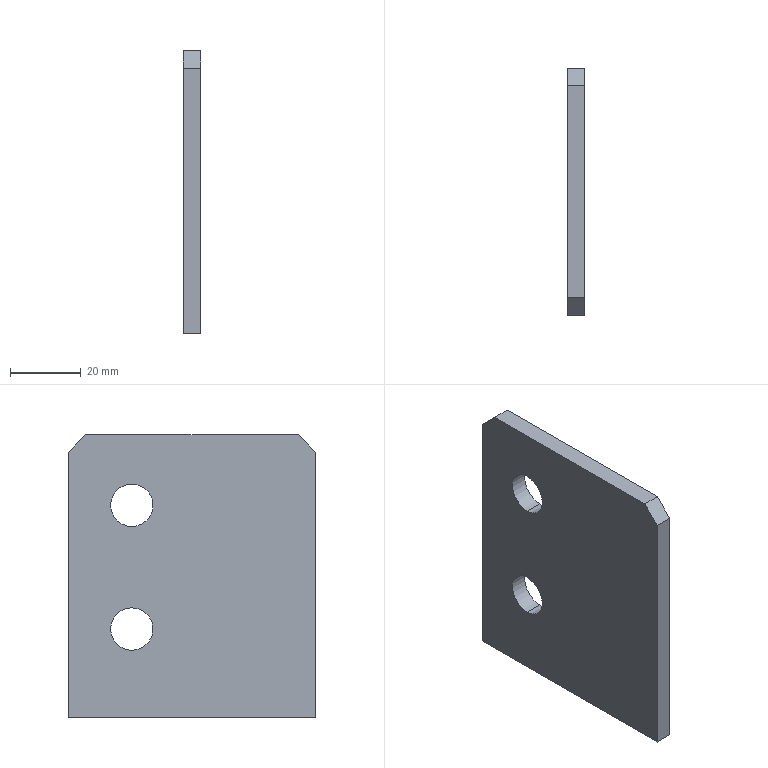Part | STEP file | 1 solid | 12 faces | box 5 x 70 x 80 mm | volume 26744 mm3 | plane 8 | cylinder 4 | commonest cylinder face diameters 12 x4
STEP:
#1=CARTESIAN_POINT('',(0.,0.,0.));
#2=DIRECTION('',(0.,0.,1.));
#3=DIRECTION('',(1.,0.,0.));
#4=AXIS2_PLACEMENT_3D('',#1,#2,#3);
#5=CARTESIAN_POINT('',(165.,97.,31.));
#6=VERTEX_POINT('',#5);
#7=CARTESIAN_POINT('',(165.,97.,19.));
#8=VERTEX_POINT('',#7);
#9=CARTESIAN_POINT('',(165.,97.,25.));
#10=DIRECTION('',(-1.,0.,0.));
#11=DIRECTION('',(0.,0.,1.));
#12=AXIS2_PLACEMENT_3D('',#9,#10,#11);
#13=CIRCLE('',#12,6.);
#14=CARTESIAN_POINT('',(165.,115.,80.));
#15=DIRECTION('',(-1.,0.,0.));
#16=DIRECTION('',(0.,0.,1.));
#17=AXIS2_PLACEMENT_3D('',#14,#15,#16);
#18=PLANE('',#17);
#19=CARTESIAN_POINT('',(-55.,-18.));
#20=DIRECTION('',(1.,0.));
#21=AXIS2_PLACEMENT_2D('',#19,#20);
#22=CIRCLE('',#21,6.);
#23=(GEOMETRIC_REPRESENTATION_CONTEXT(2)PARAMETRIC_REPRESENTATION_CONTEXT()REPRESENTATION_CONTEXT('',''));
#24=DEFINITIONAL_REPRESENTATION('',(#22),#23);
#25=PCURVE('',#18,#24);
#26=CARTESIAN_POINT('',(160.,97.,25.));
#27=DIRECTION('',(-1.,0.,0.));
#28=DIRECTION('',(0.,0.,1.));
#29=AXIS2_PLACEMENT_3D('',#26,#27,#28);
#30=CYLINDRICAL_SURFACE('',#29,6.);
#31=CARTESIAN_POINT('',(0.,-5.));
#32=DIRECTION('',(1.,0.));
#33=VECTOR('',#32,1.);
#34=LINE('',#31,#33);
#35=(GEOMETRIC_REPRESENTATION_CONTEXT(2)PARAMETRIC_REPRESENTATION_CONTEXT()REPRESENTATION_CONTEXT('',''));
#36=DEFINITIONAL_REPRESENTATION('',(#34),#35);
#37=PCURVE('',#30,#36);
#38=SURFACE_CURVE('',#13,(#25,#37),.PCURVE_S1.);
#39=EDGE_CURVE('',#6,#8,#38,.T.);
#40=ORIENTED_EDGE('',*,*,#39,.T.);
#41=CARTESIAN_POINT('',(165.,97.,25.));
#42=DIRECTION('',(-1.,0.,0.));
#43=DIRECTION('',(0.,0.,1.));
#44=AXIS2_PLACEMENT_3D('',#41,#42,#43);
#45=CIRCLE('',#44,6.);
#46=CARTESIAN_POINT('',(-55.,-18.));
#47=DIRECTION('',(1.,0.));
#48=AXIS2_PLACEMENT_2D('',#46,#47);
#49=CIRCLE('',#48,6.);
#50=(GEOMETRIC_REPRESENTATION_CONTEXT(2)PARAMETRIC_REPRESENTATION_CONTEXT()REPRESENTATION_CONTEXT('',''));
#51=DEFINITIONAL_REPRESENTATION('',(#49),#50);
#52=PCURVE('',#18,#51);
#53=CARTESIAN_POINT('',(160.,97.,25.));
#54=DIRECTION('',(-1.,0.,0.));
#55=DIRECTION('',(0.,0.,1.));
#56=AXIS2_PLACEMENT_3D('',#53,#54,#55);
#57=CYLINDRICAL_SURFACE('',#56,6.);
#58=CARTESIAN_POINT('',(0.,-5.));
#59=DIRECTION('',(1.,0.));
#60=VECTOR('',#59,1.);
#61=LINE('',#58,#60);
#62=(GEOMETRIC_REPRESENTATION_CONTEXT(2)PARAMETRIC_REPRESENTATION_CONTEXT()REPRESENTATION_CONTEXT('',''));
#63=DEFINITIONAL_REPRESENTATION('',(#61),#62);
#64=PCURVE('',#57,#63);
#65=SURFACE_CURVE('',#45,(#52,#64),.PCURVE_S1.);
#66=EDGE_CURVE('',#8,#6,#65,.T.);
#67=ORIENTED_EDGE('',*,*,#66,.T.);
#68=EDGE_LOOP('',(#40,#67));
#69=FACE_BOUND('',#68,.T.);
#70=CARTESIAN_POINT('',(165.,97.,66.));
#71=VERTEX_POINT('',#70);
#72=CARTESIAN_POINT('',(165.,97.,54.));
#73=VERTEX_POINT('',#72);
#74=CARTESIAN_POINT('',(165.,97.,60.));
#75=DIRECTION('',(-1.,0.,0.));
#76=DIRECTION('',(0.,0.,1.));
#77=AXIS2_PLACEMENT_3D('',#74,#75,#76);
#78=CIRCLE('',#77,6.);
#79=CARTESIAN_POINT('',(-20.,-18.));
#80=DIRECTION('',(1.,0.));
#81=AXIS2_PLACEMENT_2D('',#79,#80);
#82=CIRCLE('',#81,6.);
#83=(GEOMETRIC_REPRESENTATION_CONTEXT(2)PARAMETRIC_REPRESENTATION_CONTEXT()REPRESENTATION_CONTEXT('',''));
#84=DEFINITIONAL_REPRESENTATION('',(#82),#83);
#85=PCURVE('',#18,#84);
#86=CARTESIAN_POINT('',(160.,97.,60.));
#87=DIRECTION('',(-1.,0.,0.));
#88=DIRECTION('',(0.,0.,1.));
#89=AXIS2_PLACEMENT_3D('',#86,#87,#88);
#90=CYLINDRICAL_SURFACE('',#89,6.);
#91=CARTESIAN_POINT('',(0.,-5.));
#92=DIRECTION('',(1.,0.));
#93=VECTOR('',#92,1.);
#94=LINE('',#91,#93);
#95=(GEOMETRIC_REPRESENTATION_CONTEXT(2)PARAMETRIC_REPRESENTATION_CONTEXT()REPRESENTATION_CONTEXT('',''));
#96=DEFINITIONAL_REPRESENTATION('',(#94),#95);
#97=PCURVE('',#90,#96);
#98=SURFACE_CURVE('',#78,(#85,#97),.PCURVE_S1.);
#99=EDGE_CURVE('',#71,#73,#98,.T.);
#100=ORIENTED_EDGE('',*,*,#99,.T.);
#101=CARTESIAN_POINT('',(165.,97.,60.));
#102=DIRECTION('',(-1.,0.,0.));
#103=DIRECTION('',(0.,0.,1.));
#104=AXIS2_PLACEMENT_3D('',#101,#102,#103);
#105=CIRCLE('',#104,6.);
#106=CARTESIAN_POINT('',(-20.,-18.));
#107=DIRECTION('',(1.,0.));
#108=AXIS2_PLACEMENT_2D('',#106,#107);
#109=CIRCLE('',#108,6.);
#110=(GEOMETRIC_REPRESENTATION_CONTEXT(2)PARAMETRIC_REPRESENTATION_CONTEXT()REPRESENTATION_CONTEXT('',''));
#111=DEFINITIONAL_REPRESENTATION('',(#109),#110);
#112=PCURVE('',#18,#111);
#113=CARTESIAN_POINT('',(160.,97.,60.));
#114=DIRECTION('',(-1.,0.,0.));
#115=DIRECTION('',(0.,0.,1.));
#116=AXIS2_PLACEMENT_3D('',#113,#114,#115);
#117=CYLINDRICAL_SURFACE('',#116,6.);
#118=CARTESIAN_POINT('',(0.,-5.));
#119=DIRECTION('',(1.,0.));
#120=VECTOR('',#119,1.);
#121=LINE('',#118,#120);
#122=(GEOMETRIC_REPRESENTATION_CONTEXT(2)PARAMETRIC_REPRESENTATION_CONTEXT()REPRESENTATION_CONTEXT('',''));
#123=DEFINITIONAL_REPRESENTATION('',(#121),#122);
#124=PCURVE('',#117,#123);
#125=SURFACE_CURVE('',#105,(#112,#124),.PCURVE_S1.);
#126=EDGE_CURVE('',#73,#71,#125,.T.);
#127=ORIENTED_EDGE('',*,*,#126,.T.);
#128=EDGE_LOOP('',(#100,#127));
#129=FACE_BOUND('',#128,.T.);
#130=CARTESIAN_POINT('',(165.,45.,75.));
#131=VERTEX_POINT('',#130);
#132=CARTESIAN_POINT('',(165.,50.,80.));
#133=VERTEX_POINT('',#132);
#134=CARTESIAN_POINT('',(165.,50.,80.));
#135=DIRECTION('',(0.,0.7071,0.7071));
#136=VECTOR('',#135,1.);
#137=LINE('',#134,#136);
#138=CARTESIAN_POINT('',(0.,-65.));
#139=DIRECTION('',(0.7071,0.7071));
#140=VECTOR('',#139,1.);
#141=LINE('',#138,#140);
#142=(GEOMETRIC_REPRESENTATION_CONTEXT(2)PARAMETRIC_REPRESENTATION_CONTEXT()REPRESENTATION_CONTEXT('',''));
#143=DEFINITIONAL_REPRESENTATION('',(#141),#142);
#144=PCURVE('',#18,#143);
#145=CARTESIAN_POINT('',(0.,50.,80.));
#146=DIRECTION('',(0.,-0.7071,0.7071));
#147=DIRECTION('',(-1.,0.,0.));
#148=AXIS2_PLACEMENT_3D('',#145,#146,#147);
#149=PLANE('',#148);
#150=CARTESIAN_POINT('',(-165.,0.));
#151=DIRECTION('',(0.,-1.));
#152=VECTOR('',#151,1.);
#153=LINE('',#150,#152);
#154=(GEOMETRIC_REPRESENTATION_CONTEXT(2)PARAMETRIC_REPRESENTATION_CONTEXT()REPRESENTATION_CONTEXT('',''));
#155=DEFINITIONAL_REPRESENTATION('',(#153),#154);
#156=PCURVE('',#149,#155);
#157=SURFACE_CURVE('',#137,(#144,#156),.PCURVE_S1.);
#158=EDGE_CURVE('',#131,#133,#157,.T.);
#159=ORIENTED_EDGE('',*,*,#158,.F.);
#160=CARTESIAN_POINT('',(165.,45.,0.));
#161=VERTEX_POINT('',#160);
#162=CARTESIAN_POINT('',(165.,45.,80.));
#163=DIRECTION('',(0.,0.,-1.));
#164=VECTOR('',#163,1.);
#165=LINE('',#162,#164);
#166=CARTESIAN_POINT('',(0.,-70.));
#167=DIRECTION('',(-1.,0.));
#168=VECTOR('',#167,1.);
#169=LINE('',#166,#168);
#170=(GEOMETRIC_REPRESENTATION_CONTEXT(2)PARAMETRIC_REPRESENTATION_CONTEXT()REPRESENTATION_CONTEXT('',''));
#171=DEFINITIONAL_REPRESENTATION('',(#169),#170);
#172=PCURVE('',#18,#171);
#173=CARTESIAN_POINT('',(160.,45.,80.));
#174=DIRECTION('',(0.,1.,0.));
#175=DIRECTION('',(1.,0.,0.));
#176=AXIS2_PLACEMENT_3D('',#173,#174,#175);
#177=PLANE('',#176);
#178=CARTESIAN_POINT('',(5.,0.));
#179=DIRECTION('',(0.,1.));
#180=VECTOR('',#179,1.);
#181=LINE('',#178,#180);
#182=(GEOMETRIC_REPRESENTATION_CONTEXT(2)PARAMETRIC_REPRESENTATION_CONTEXT()REPRESENTATION_CONTEXT('',''));
#183=DEFINITIONAL_REPRESENTATION('',(#181),#182);
#184=PCURVE('',#177,#183);
#185=SURFACE_CURVE('',#165,(#172,#184),.PCURVE_S1.);
#186=EDGE_CURVE('',#131,#161,#185,.T.);
#187=ORIENTED_EDGE('',*,*,#186,.T.);
#188=CARTESIAN_POINT('',(165.,115.,0.));
#189=VERTEX_POINT('',#188);
#190=CARTESIAN_POINT('',(165.,0.,0.));
#191=DIRECTION('',(0.,1.,0.));
#192=VECTOR('',#191,1.);
#193=LINE('',#190,#192);
#194=CARTESIAN_POINT('',(-80.,-115.));
#195=DIRECTION('',(0.,1.));
#196=VECTOR('',#195,1.);
#197=LINE('',#194,#196);
#198=(GEOMETRIC_REPRESENTATION_CONTEXT(2)PARAMETRIC_REPRESENTATION_CONTEXT()REPRESENTATION_CONTEXT('',''));
#199=DEFINITIONAL_REPRESENTATION('',(#197),#198);
#200=PCURVE('',#18,#199);
#201=CARTESIAN_POINT('',(0.,0.,0.));
#202=DIRECTION('',(0.,0.,1.));
#203=DIRECTION('',(1.,0.,0.));
#204=AXIS2_PLACEMENT_3D('',#201,#202,#203);
#205=PLANE('',#204);
#206=CARTESIAN_POINT('',(165.,0.));
#207=DIRECTION('',(0.,1.));
#208=VECTOR('',#207,1.);
#209=LINE('',#206,#208);
#210=(GEOMETRIC_REPRESENTATION_CONTEXT(2)PARAMETRIC_REPRESENTATION_CONTEXT()REPRESENTATION_CONTEXT('',''));
#211=DEFINITIONAL_REPRESENTATION('',(#209),#210);
#212=PCURVE('',#205,#211);
#213=SURFACE_CURVE('',#193,(#200,#212),.PCURVE_S1.);
#214=EDGE_CURVE('',#161,#189,#213,.T.);
#215=ORIENTED_EDGE('',*,*,#214,.T.);
#216=CARTESIAN_POINT('',(165.,115.,75.));
#217=VERTEX_POINT('',#216);
#218=CARTESIAN_POINT('',(165.,115.,80.));
#219=DIRECTION('',(0.,0.,1.));
#220=VECTOR('',#219,1.);
#221=LINE('',#218,#220);
#222=CARTESIAN_POINT('',(0.,0.));
#223=DIRECTION('',(1.,0.));
#224=VECTOR('',#223,1.);
#225=LINE('',#222,#224);
#226=(GEOMETRIC_REPRESENTATION_CONTEXT(2)PARAMETRIC_REPRESENTATION_CONTEXT()REPRESENTATION_CONTEXT('',''));
#227=DEFINITIONAL_REPRESENTATION('',(#225),#226);
#228=PCURVE('',#18,#227);
#229=CARTESIAN_POINT('',(160.,115.,80.));
#230=DIRECTION('',(0.,-1.,0.));
#231=DIRECTION('',(0.,0.,-1.));
#232=AXIS2_PLACEMENT_3D('',#229,#230,#231);
#233=PLANE('',#232);
#234=CARTESIAN_POINT('',(0.,5.));
#235=DIRECTION('',(-1.,0.));
#236=VECTOR('',#235,1.);
#237=LINE('',#234,#236);
#238=(GEOMETRIC_REPRESENTATION_CONTEXT(2)PARAMETRIC_REPRESENTATION_CONTEXT()REPRESENTATION_CONTEXT('',''));
#239=DEFINITIONAL_REPRESENTATION('',(#237),#238);
#240=PCURVE('',#233,#239);
#241=SURFACE_CURVE('',#221,(#228,#240),.PCURVE_S1.);
#242=EDGE_CURVE('',#189,#217,#241,.T.);
#243=ORIENTED_EDGE('',*,*,#242,.T.);
#244=CARTESIAN_POINT('',(165.,110.,80.));
#245=VERTEX_POINT('',#244);
#246=CARTESIAN_POINT('',(165.,110.,80.));
#247=DIRECTION('',(0.,0.7071,-0.7071));
#248=VECTOR('',#247,1.);
#249=LINE('',#246,#248);
#250=CARTESIAN_POINT('',(0.,-5.));
#251=DIRECTION('',(-0.7071,0.7071));
#252=VECTOR('',#251,1.);
#253=LINE('',#250,#252);
#254=(GEOMETRIC_REPRESENTATION_CONTEXT(2)PARAMETRIC_REPRESENTATION_CONTEXT()REPRESENTATION_CONTEXT('',''));
#255=DEFINITIONAL_REPRESENTATION('',(#253),#254);
#256=PCURVE('',#18,#255);
#257=CARTESIAN_POINT('',(0.,110.,80.));
#258=DIRECTION('',(0.,0.7071,0.7071));
#259=DIRECTION('',(1.,0.,0.));
#260=AXIS2_PLACEMENT_3D('',#257,#258,#259);
#261=PLANE('',#260);
#262=CARTESIAN_POINT('',(165.,0.));
#263=DIRECTION('',(0.,1.));
#264=VECTOR('',#263,1.);
#265=LINE('',#262,#264);
#266=(GEOMETRIC_REPRESENTATION_CONTEXT(2)PARAMETRIC_REPRESENTATION_CONTEXT()REPRESENTATION_CONTEXT('',''));
#267=DEFINITIONAL_REPRESENTATION('',(#265),#266);
#268=PCURVE('',#261,#267);
#269=SURFACE_CURVE('',#249,(#256,#268),.PCURVE_S1.);
#270=EDGE_CURVE('',#245,#217,#269,.T.);
#271=ORIENTED_EDGE('',*,*,#270,.F.);
#272=CARTESIAN_POINT('',(165.,0.,80.));
#273=DIRECTION('',(0.,1.,0.));
#274=VECTOR('',#273,1.);
#275=LINE('',#272,#274);
#276=CARTESIAN_POINT('',(0.,-115.));
#277=DIRECTION('',(0.,1.));
#278=VECTOR('',#277,1.);
#279=LINE('',#276,#278);
#280=(GEOMETRIC_REPRESENTATION_CONTEXT(2)PARAMETRIC_REPRESENTATION_CONTEXT()REPRESENTATION_CONTEXT('',''));
#281=DEFINITIONAL_REPRESENTATION('',(#279),#280);
#282=PCURVE('',#18,#281);
#283=CARTESIAN_POINT('',(0.,0.,80.));
#284=DIRECTION('',(0.,0.,1.));
#285=DIRECTION('',(1.,0.,0.));
#286=AXIS2_PLACEMENT_3D('',#283,#284,#285);
#287=PLANE('',#286);
#288=CARTESIAN_POINT('',(165.,0.));
#289=DIRECTION('',(0.,1.));
#290=VECTOR('',#289,1.);
#291=LINE('',#288,#290);
#292=(GEOMETRIC_REPRESENTATION_CONTEXT(2)PARAMETRIC_REPRESENTATION_CONTEXT()REPRESENTATION_CONTEXT('',''));
#293=DEFINITIONAL_REPRESENTATION('',(#291),#292);
#294=PCURVE('',#287,#293);
#295=SURFACE_CURVE('',#275,(#282,#294),.PCURVE_S1.);
#296=EDGE_CURVE('',#133,#245,#295,.T.);
#297=ORIENTED_EDGE('',*,*,#296,.F.);
#298=EDGE_LOOP('',(#159,#187,#215,#243,#271,#297));
#299=FACE_BOUND('',#298,.T.);
#300=ADVANCED_FACE('',(#69,#129,#299),#18,.F.);
#301=CARTESIAN_POINT('',(160.,97.,31.));
#302=VERTEX_POINT('',#301);
#303=CARTESIAN_POINT('',(160.,97.,19.));
#304=VERTEX_POINT('',#303);
#305=CARTESIAN_POINT('',(160.,97.,25.));
#306=DIRECTION('',(-1.,0.,0.));
#307=DIRECTION('',(0.,0.,1.));
#308=AXIS2_PLACEMENT_3D('',#305,#306,#307);
#309=CIRCLE('',#308,6.);
#310=CARTESIAN_POINT('',(0.,0.));
#311=DIRECTION('',(1.,0.));
#312=VECTOR('',#311,1.);
#313=LINE('',#310,#312);
#314=(GEOMETRIC_REPRESENTATION_CONTEXT(2)PARAMETRIC_REPRESENTATION_CONTEXT()REPRESENTATION_CONTEXT('',''));
#315=DEFINITIONAL_REPRESENTATION('',(#313),#314);
#316=PCURVE('',#30,#315);
#317=CARTESIAN_POINT('',(160.,115.,80.));
#318=DIRECTION('',(1.,0.,0.));
#319=DIRECTION('',(0.,1.,0.));
#320=AXIS2_PLACEMENT_3D('',#317,#318,#319);
#321=PLANE('',#320);
#322=CARTESIAN_POINT('',(-18.,-49.));
#323=CARTESIAN_POINT('',(-7.608,-49.));
#324=CARTESIAN_POINT('',(-12.804,-58.));
#325=CARTESIAN_POINT('',(-18.,-67.));
#326=CARTESIAN_POINT('',(-23.196,-58.));
#327=CARTESIAN_POINT('',(-28.392,-49.));
#328=CARTESIAN_POINT('',(-18.,-49.));
#329=(BOUNDED_CURVE()B_SPLINE_CURVE(2,(#322,#323,#324,#325,#326,#327,#328),.UNSPECIFIED.,.T.,.F.)B_SPLINE_CURVE_WITH_KNOTS((1,2,2,2,2,1),(-2.094,0.,2.094,4.189,6.283,8.378),.UNSPECIFIED.)CURVE()GEOMETRIC_REPRESENTATION_ITEM()RATIONAL_B_SPLINE_CURVE((1.,0.5,1.,0.5,1.,0.5,1.))REPRESENTATION_ITEM(''));
#330=(GEOMETRIC_REPRESENTATION_CONTEXT(2)PARAMETRIC_REPRESENTATION_CONTEXT()REPRESENTATION_CONTEXT('',''));
#331=DEFINITIONAL_REPRESENTATION('',(#329),#330);
#332=PCURVE('',#321,#331);
#333=SURFACE_CURVE('',#309,(#316,#332),.PCURVE_S1.);
#334=EDGE_CURVE('',#302,#304,#333,.T.);
#335=ORIENTED_EDGE('',*,*,#334,.F.);
#336=CARTESIAN_POINT('',(160.,97.,31.));
#337=DIRECTION('',(-1.,0.,0.));
#338=VECTOR('',#337,1.);
#339=LINE('',#336,#338);
#340=CARTESIAN_POINT('',(0.,0.));
#341=DIRECTION('',(0.,1.));
#342=VECTOR('',#341,1.);
#343=LINE('',#340,#342);
#344=(GEOMETRIC_REPRESENTATION_CONTEXT(2)PARAMETRIC_REPRESENTATION_CONTEXT()REPRESENTATION_CONTEXT('',''));
#345=DEFINITIONAL_REPRESENTATION('',(#343),#344);
#346=PCURVE('',#30,#345);
#347=CARTESIAN_POINT('',(6.283,0.));
#348=DIRECTION('',(0.,1.));
#349=VECTOR('',#348,1.);
#350=LINE('',#347,#349);
#351=(GEOMETRIC_REPRESENTATION_CONTEXT(2)PARAMETRIC_REPRESENTATION_CONTEXT()REPRESENTATION_CONTEXT('',''));
#352=DEFINITIONAL_REPRESENTATION('',(#350),#351);
#353=PCURVE('',#57,#352);
#354=SURFACE_CURVE('',#339,(#346,#353),.PCURVE_S1.);
#355=EDGE_CURVE('',#6,#302,#354,.T.);
#356=ORIENTED_EDGE('',*,*,#355,.F.);
#357=ORIENTED_EDGE('',*,*,#39,.T.);
#358=CARTESIAN_POINT('',(160.,97.,19.));
#359=DIRECTION('',(-1.,0.,0.));
#360=VECTOR('',#359,1.);
#361=LINE('',#358,#360);
#362=CARTESIAN_POINT('',(3.142,0.));
#363=DIRECTION('',(0.,1.));
#364=VECTOR('',#363,1.);
#365=LINE('',#362,#364);
#366=(GEOMETRIC_REPRESENTATION_CONTEXT(2)PARAMETRIC_REPRESENTATION_CONTEXT()REPRESENTATION_CONTEXT('',''));
#367=DEFINITIONAL_REPRESENTATION('',(#365),#366);
#368=PCURVE('',#30,#367);
#369=CARTESIAN_POINT('',(3.142,0.));
#370=DIRECTION('',(0.,1.));
#371=VECTOR('',#370,1.);
#372=LINE('',#369,#371);
#373=(GEOMETRIC_REPRESENTATION_CONTEXT(2)PARAMETRIC_REPRESENTATION_CONTEXT()REPRESENTATION_CONTEXT('',''));
#374=DEFINITIONAL_REPRESENTATION('',(#372),#373);
#375=PCURVE('',#57,#374);
#376=SURFACE_CURVE('',#361,(#368,#375),.PCURVE_S1.);
#377=EDGE_CURVE('',#8,#304,#376,.T.);
#378=ORIENTED_EDGE('',*,*,#377,.T.);
#379=EDGE_LOOP('',(#335,#356,#357,#378));
#380=FACE_BOUND('',#379,.F.);
#381=ADVANCED_FACE('',(#380),#30,.F.);
#382=CARTESIAN_POINT('',(160.,97.,66.));
#383=VERTEX_POINT('',#382);
#384=CARTESIAN_POINT('',(160.,97.,54.));
#385=VERTEX_POINT('',#384);
#386=CARTESIAN_POINT('',(160.,97.,60.));
#387=DIRECTION('',(-1.,0.,0.));
#388=DIRECTION('',(0.,0.,1.));
#389=AXIS2_PLACEMENT_3D('',#386,#387,#388);
#390=CIRCLE('',#389,6.);
#391=CARTESIAN_POINT('',(0.,0.));
#392=DIRECTION('',(1.,0.));
#393=VECTOR('',#392,1.);
#394=LINE('',#391,#393);
#395=(GEOMETRIC_REPRESENTATION_CONTEXT(2)PARAMETRIC_REPRESENTATION_CONTEXT()REPRESENTATION_CONTEXT('',''));
#396=DEFINITIONAL_REPRESENTATION('',(#394),#395);
#397=PCURVE('',#90,#396);
#398=CARTESIAN_POINT('',(-18.,-14.));
#399=CARTESIAN_POINT('',(-7.608,-14.));
#400=CARTESIAN_POINT('',(-12.804,-23.));
#401=CARTESIAN_POINT('',(-18.,-32.));
#402=CARTESIAN_POINT('',(-23.196,-23.));
#403=CARTESIAN_POINT('',(-28.392,-14.));
#404=CARTESIAN_POINT('',(-18.,-14.));
#405=(BOUNDED_CURVE()B_SPLINE_CURVE(2,(#398,#399,#400,#401,#402,#403,#404),.UNSPECIFIED.,.T.,.F.)B_SPLINE_CURVE_WITH_KNOTS((1,2,2,2,2,1),(-2.094,0.,2.094,4.189,6.283,8.378),.UNSPECIFIED.)CURVE()GEOMETRIC_REPRESENTATION_ITEM()RATIONAL_B_SPLINE_CURVE((1.,0.5,1.,0.5,1.,0.5,1.))REPRESENTATION_ITEM(''));
#406=(GEOMETRIC_REPRESENTATION_CONTEXT(2)PARAMETRIC_REPRESENTATION_CONTEXT()REPRESENTATION_CONTEXT('',''));
#407=DEFINITIONAL_REPRESENTATION('',(#405),#406);
#408=PCURVE('',#321,#407);
#409=SURFACE_CURVE('',#390,(#397,#408),.PCURVE_S1.);
#410=EDGE_CURVE('',#383,#385,#409,.T.);
#411=ORIENTED_EDGE('',*,*,#410,.F.);
#412=CARTESIAN_POINT('',(160.,97.,66.));
#413=DIRECTION('',(-1.,0.,0.));
#414=VECTOR('',#413,1.);
#415=LINE('',#412,#414);
#416=CARTESIAN_POINT('',(0.,0.));
#417=DIRECTION('',(0.,1.));
#418=VECTOR('',#417,1.);
#419=LINE('',#416,#418);
#420=(GEOMETRIC_REPRESENTATION_CONTEXT(2)PARAMETRIC_REPRESENTATION_CONTEXT()REPRESENTATION_CONTEXT('',''));
#421=DEFINITIONAL_REPRESENTATION('',(#419),#420);
#422=PCURVE('',#90,#421);
#423=CARTESIAN_POINT('',(6.283,0.));
#424=DIRECTION('',(0.,1.));
#425=VECTOR('',#424,1.);
#426=LINE('',#423,#425);
#427=(GEOMETRIC_REPRESENTATION_CONTEXT(2)PARAMETRIC_REPRESENTATION_CONTEXT()REPRESENTATION_CONTEXT('',''));
#428=DEFINITIONAL_REPRESENTATION('',(#426),#427);
#429=PCURVE('',#117,#428);
#430=SURFACE_CURVE('',#415,(#422,#429),.PCURVE_S1.);
#431=EDGE_CURVE('',#71,#383,#430,.T.);
#432=ORIENTED_EDGE('',*,*,#431,.F.);
#433=ORIENTED_EDGE('',*,*,#99,.T.);
#434=CARTESIAN_POINT('',(160.,97.,54.));
#435=DIRECTION('',(-1.,0.,0.));
#436=VECTOR('',#435,1.);
#437=LINE('',#434,#436);
#438=CARTESIAN_POINT('',(3.142,0.));
#439=DIRECTION('',(0.,1.));
#440=VECTOR('',#439,1.);
#441=LINE('',#438,#440);
#442=(GEOMETRIC_REPRESENTATION_CONTEXT(2)PARAMETRIC_REPRESENTATION_CONTEXT()REPRESENTATION_CONTEXT('',''));
#443=DEFINITIONAL_REPRESENTATION('',(#441),#442);
#444=PCURVE('',#90,#443);
#445=CARTESIAN_POINT('',(3.142,0.));
#446=DIRECTION('',(0.,1.));
#447=VECTOR('',#446,1.);
#448=LINE('',#445,#447);
#449=(GEOMETRIC_REPRESENTATION_CONTEXT(2)PARAMETRIC_REPRESENTATION_CONTEXT()REPRESENTATION_CONTEXT('',''));
#450=DEFINITIONAL_REPRESENTATION('',(#448),#449);
#451=PCURVE('',#117,#450);
#452=SURFACE_CURVE('',#437,(#444,#451),.PCURVE_S1.);
#453=EDGE_CURVE('',#73,#385,#452,.T.);
#454=ORIENTED_EDGE('',*,*,#453,.T.);
#455=EDGE_LOOP('',(#411,#432,#433,#454));
#456=FACE_BOUND('',#455,.F.);
#457=ADVANCED_FACE('',(#456),#90,.F.);
#458=CARTESIAN_POINT('',(160.,115.,0.));
#459=VERTEX_POINT('',#458);
#460=CARTESIAN_POINT('',(160.,115.,0.));
#461=DIRECTION('',(1.,0.,0.));
#462=VECTOR('',#461,1.);
#463=LINE('',#460,#462);
#464=CARTESIAN_POINT('',(160.,115.));
#465=DIRECTION('',(1.,0.));
#466=VECTOR('',#465,1.);
#467=LINE('',#464,#466);
#468=(GEOMETRIC_REPRESENTATION_CONTEXT(2)PARAMETRIC_REPRESENTATION_CONTEXT()REPRESENTATION_CONTEXT('',''));
#469=DEFINITIONAL_REPRESENTATION('',(#467),#468);
#470=PCURVE('',#205,#469);
#471=CARTESIAN_POINT('',(80.,0.));
#472=DIRECTION('',(0.,1.));
#473=VECTOR('',#472,1.);
#474=LINE('',#471,#473);
#475=(GEOMETRIC_REPRESENTATION_CONTEXT(2)PARAMETRIC_REPRESENTATION_CONTEXT()REPRESENTATION_CONTEXT('',''));
#476=DEFINITIONAL_REPRESENTATION('',(#474),#475);
#477=PCURVE('',#233,#476);
#478=SURFACE_CURVE('',#463,(#470,#477),.PCURVE_S1.);
#479=EDGE_CURVE('',#459,#189,#478,.T.);
#480=ORIENTED_EDGE('',*,*,#479,.T.);
#481=ORIENTED_EDGE('',*,*,#214,.F.);
#482=CARTESIAN_POINT('',(160.,45.,0.));
#483=VERTEX_POINT('',#482);
#484=CARTESIAN_POINT('',(160.,45.,0.));
#485=DIRECTION('',(-1.,0.,0.));
#486=VECTOR('',#485,1.);
#487=LINE('',#484,#486);
#488=CARTESIAN_POINT('',(160.,45.));
#489=DIRECTION('',(-1.,0.));
#490=VECTOR('',#489,1.);
#491=LINE('',#488,#490);
#492=(GEOMETRIC_REPRESENTATION_CONTEXT(2)PARAMETRIC_REPRESENTATION_CONTEXT()REPRESENTATION_CONTEXT('',''));
#493=DEFINITIONAL_REPRESENTATION('',(#491),#492);
#494=PCURVE('',#205,#493);
#495=CARTESIAN_POINT('',(0.,80.));
#496=DIRECTION('',(-1.,0.));
#497=VECTOR('',#496,1.);
#498=LINE('',#495,#497);
#499=(GEOMETRIC_REPRESENTATION_CONTEXT(2)PARAMETRIC_REPRESENTATION_CONTEXT()REPRESENTATION_CONTEXT('',''));
#500=DEFINITIONAL_REPRESENTATION('',(#498),#499);
#501=PCURVE('',#177,#500);
#502=SURFACE_CURVE('',#487,(#494,#501),.PCURVE_S1.);
#503=EDGE_CURVE('',#161,#483,#502,.T.);
#504=ORIENTED_EDGE('',*,*,#503,.T.);
#505=CARTESIAN_POINT('',(160.,115.,0.));
#506=DIRECTION('',(0.,1.,0.));
#507=VECTOR('',#506,1.);
#508=LINE('',#505,#507);
#509=CARTESIAN_POINT('',(160.,115.));
#510=DIRECTION('',(0.,1.));
#511=VECTOR('',#510,1.);
#512=LINE('',#509,#511);
#513=(GEOMETRIC_REPRESENTATION_CONTEXT(2)PARAMETRIC_REPRESENTATION_CONTEXT()REPRESENTATION_CONTEXT('',''));
#514=DEFINITIONAL_REPRESENTATION('',(#512),#513);
#515=PCURVE('',#205,#514);
#516=CARTESIAN_POINT('',(0.,-80.));
#517=DIRECTION('',(1.,0.));
#518=VECTOR('',#517,1.);
#519=LINE('',#516,#518);
#520=(GEOMETRIC_REPRESENTATION_CONTEXT(2)PARAMETRIC_REPRESENTATION_CONTEXT()REPRESENTATION_CONTEXT('',''));
#521=DEFINITIONAL_REPRESENTATION('',(#519),#520);
#522=PCURVE('',#321,#521);
#523=SURFACE_CURVE('',#508,(#515,#522),.PCURVE_S1.);
#524=EDGE_CURVE('',#483,#459,#523,.T.);
#525=ORIENTED_EDGE('',*,*,#524,.T.);
#526=EDGE_LOOP('',(#480,#481,#504,#525));
#527=FACE_BOUND('',#526,.T.);
#528=ADVANCED_FACE('',(#527),#205,.F.);
#529=CARTESIAN_POINT('',(160.,115.,75.));
#530=VERTEX_POINT('',#529);
#531=CARTESIAN_POINT('',(0.,115.,75.));
#532=DIRECTION('',(-1.,0.,0.));
#533=VECTOR('',#532,1.);
#534=LINE('',#531,#533);
#535=CARTESIAN_POINT('',(5.,-160.));
#536=DIRECTION('',(0.,-1.));
#537=VECTOR('',#536,1.);
#538=LINE('',#535,#537);
#539=(GEOMETRIC_REPRESENTATION_CONTEXT(2)PARAMETRIC_REPRESENTATION_CONTEXT()REPRESENTATION_CONTEXT('',''));
#540=DEFINITIONAL_REPRESENTATION('',(#538),#539);
#541=PCURVE('',#233,#540);
#542=CARTESIAN_POINT('',(0.,7.071));
#543=DIRECTION('',(-1.,0.));
#544=VECTOR('',#543,1.);
#545=LINE('',#542,#544);
#546=(GEOMETRIC_REPRESENTATION_CONTEXT(2)PARAMETRIC_REPRESENTATION_CONTEXT()REPRESENTATION_CONTEXT('',''));
#547=DEFINITIONAL_REPRESENTATION('',(#545),#546);
#548=PCURVE('',#261,#547);
#549=SURFACE_CURVE('',#534,(#541,#548),.PCURVE_S1.);
#550=EDGE_CURVE('',#217,#530,#549,.T.);
#551=ORIENTED_EDGE('',*,*,#550,.F.);
#552=ORIENTED_EDGE('',*,*,#242,.F.);
#553=ORIENTED_EDGE('',*,*,#479,.F.);
#554=CARTESIAN_POINT('',(160.,115.,80.));
#555=DIRECTION('',(0.,0.,1.));
#556=VECTOR('',#555,1.);
#557=LINE('',#554,#556);
#558=CARTESIAN_POINT('',(0.,0.));
#559=DIRECTION('',(-1.,0.));
#560=VECTOR('',#559,1.);
#561=LINE('',#558,#560);
#562=(GEOMETRIC_REPRESENTATION_CONTEXT(2)PARAMETRIC_REPRESENTATION_CONTEXT()REPRESENTATION_CONTEXT('',''));
#563=DEFINITIONAL_REPRESENTATION('',(#561),#562);
#564=PCURVE('',#233,#563);
#565=CARTESIAN_POINT('',(0.,0.));
#566=DIRECTION('',(0.,1.));
#567=VECTOR('',#566,1.);
#568=LINE('',#565,#567);
#569=(GEOMETRIC_REPRESENTATION_CONTEXT(2)PARAMETRIC_REPRESENTATION_CONTEXT()REPRESENTATION_CONTEXT('',''));
#570=DEFINITIONAL_REPRESENTATION('',(#568),#569);
#571=PCURVE('',#321,#570);
#572=SURFACE_CURVE('',#557,(#564,#571),.PCURVE_S1.);
#573=EDGE_CURVE('',#459,#530,#572,.T.);
#574=ORIENTED_EDGE('',*,*,#573,.T.);
#575=EDGE_LOOP('',(#551,#552,#553,#574));
#576=FACE_BOUND('',#575,.T.);
#577=ADVANCED_FACE('',(#576),#233,.F.);
#578=CARTESIAN_POINT('',(160.,110.,80.));
#579=VERTEX_POINT('',#578);
#580=CARTESIAN_POINT('',(160.,115.,75.));
#581=DIRECTION('',(0.,-0.7071,0.7071));
#582=VECTOR('',#581,1.);
#583=LINE('',#580,#582);
#584=CARTESIAN_POINT('',(160.,7.071));
#585=DIRECTION('',(0.,-1.));
#586=VECTOR('',#585,1.);
#587=LINE('',#584,#586);
#588=(GEOMETRIC_REPRESENTATION_CONTEXT(2)PARAMETRIC_REPRESENTATION_CONTEXT()REPRESENTATION_CONTEXT('',''));
#589=DEFINITIONAL_REPRESENTATION('',(#587),#588);
#590=PCURVE('',#261,#589);
#591=CARTESIAN_POINT('',(0.,-5.));
#592=DIRECTION('',(-0.7071,0.7071));
#593=VECTOR('',#592,1.);
#594=LINE('',#591,#593);
#595=(GEOMETRIC_REPRESENTATION_CONTEXT(2)PARAMETRIC_REPRESENTATION_CONTEXT()REPRESENTATION_CONTEXT('',''));
#596=DEFINITIONAL_REPRESENTATION('',(#594),#595);
#597=PCURVE('',#321,#596);
#598=SURFACE_CURVE('',#583,(#590,#597),.PCURVE_S1.);
#599=EDGE_CURVE('',#530,#579,#598,.T.);
#600=ORIENTED_EDGE('',*,*,#599,.T.);
#601=CARTESIAN_POINT('',(0.,110.,80.));
#602=DIRECTION('',(-1.,0.,0.));
#603=VECTOR('',#602,1.);
#604=LINE('',#601,#603);
#605=CARTESIAN_POINT('',(0.,0.));
#606=DIRECTION('',(-1.,0.));
#607=VECTOR('',#606,1.);
#608=LINE('',#605,#607);
#609=(GEOMETRIC_REPRESENTATION_CONTEXT(2)PARAMETRIC_REPRESENTATION_CONTEXT()REPRESENTATION_CONTEXT('',''));
#610=DEFINITIONAL_REPRESENTATION('',(#608),#609);
#611=PCURVE('',#261,#610);
#612=CARTESIAN_POINT('',(0.,110.));
#613=DIRECTION('',(-1.,0.));
#614=VECTOR('',#613,1.);
#615=LINE('',#612,#614);
#616=(GEOMETRIC_REPRESENTATION_CONTEXT(2)PARAMETRIC_REPRESENTATION_CONTEXT()REPRESENTATION_CONTEXT('',''));
#617=DEFINITIONAL_REPRESENTATION('',(#615),#616);
#618=PCURVE('',#287,#617);
#619=SURFACE_CURVE('',#604,(#611,#618),.PCURVE_S1.);
#620=EDGE_CURVE('',#245,#579,#619,.T.);
#621=ORIENTED_EDGE('',*,*,#620,.F.);
#622=ORIENTED_EDGE('',*,*,#270,.T.);
#623=ORIENTED_EDGE('',*,*,#550,.T.);
#624=EDGE_LOOP('',(#600,#621,#622,#623));
#625=FACE_BOUND('',#624,.T.);
#626=ADVANCED_FACE('',(#625),#261,.T.);
#627=ORIENTED_EDGE('',*,*,#296,.T.);
#628=ORIENTED_EDGE('',*,*,#620,.T.);
#629=CARTESIAN_POINT('',(160.,50.,80.));
#630=VERTEX_POINT('',#629);
#631=CARTESIAN_POINT('',(160.,115.,80.));
#632=DIRECTION('',(0.,-1.,0.));
#633=VECTOR('',#632,1.);
#634=LINE('',#631,#633);
#635=CARTESIAN_POINT('',(160.,115.));
#636=DIRECTION('',(0.,-1.));
#637=VECTOR('',#636,1.);
#638=LINE('',#635,#637);
#639=(GEOMETRIC_REPRESENTATION_CONTEXT(2)PARAMETRIC_REPRESENTATION_CONTEXT()REPRESENTATION_CONTEXT('',''));
#640=DEFINITIONAL_REPRESENTATION('',(#638),#639);
#641=PCURVE('',#287,#640);
#642=CARTESIAN_POINT('',(0.,0.));
#643=DIRECTION('',(-1.,0.));
#644=VECTOR('',#643,1.);
#645=LINE('',#642,#644);
#646=(GEOMETRIC_REPRESENTATION_CONTEXT(2)PARAMETRIC_REPRESENTATION_CONTEXT()REPRESENTATION_CONTEXT('',''));
#647=DEFINITIONAL_REPRESENTATION('',(#645),#646);
#648=PCURVE('',#321,#647);
#649=SURFACE_CURVE('',#634,(#641,#648),.PCURVE_S1.);
#650=EDGE_CURVE('',#579,#630,#649,.T.);
#651=ORIENTED_EDGE('',*,*,#650,.T.);
#652=CARTESIAN_POINT('',(0.,50.,80.));
#653=DIRECTION('',(-1.,0.,0.));
#654=VECTOR('',#653,1.);
#655=LINE('',#652,#654);
#656=CARTESIAN_POINT('',(0.,50.));
#657=DIRECTION('',(-1.,0.));
#658=VECTOR('',#657,1.);
#659=LINE('',#656,#658);
#660=(GEOMETRIC_REPRESENTATION_CONTEXT(2)PARAMETRIC_REPRESENTATION_CONTEXT()REPRESENTATION_CONTEXT('',''));
#661=DEFINITIONAL_REPRESENTATION('',(#659),#660);
#662=PCURVE('',#287,#661);
#663=CARTESIAN_POINT('',(0.,0.));
#664=DIRECTION('',(1.,0.));
#665=VECTOR('',#664,1.);
#666=LINE('',#663,#665);
#667=(GEOMETRIC_REPRESENTATION_CONTEXT(2)PARAMETRIC_REPRESENTATION_CONTEXT()REPRESENTATION_CONTEXT('',''));
#668=DEFINITIONAL_REPRESENTATION('',(#666),#667);
#669=PCURVE('',#149,#668);
#670=SURFACE_CURVE('',#655,(#662,#669),.PCURVE_S1.);
#671=EDGE_CURVE('',#133,#630,#670,.T.);
#672=ORIENTED_EDGE('',*,*,#671,.F.);
#673=EDGE_LOOP('',(#627,#628,#651,#672));
#674=FACE_BOUND('',#673,.T.);
#675=ADVANCED_FACE('',(#674),#287,.T.);
#676=ORIENTED_EDGE('',*,*,#158,.T.);
#677=ORIENTED_EDGE('',*,*,#671,.T.);
#678=CARTESIAN_POINT('',(160.,45.,75.));
#679=VERTEX_POINT('',#678);
#680=CARTESIAN_POINT('',(160.,50.,80.));
#681=DIRECTION('',(0.,-0.7071,-0.7071));
#682=VECTOR('',#681,1.);
#683=LINE('',#680,#682);
#684=CARTESIAN_POINT('',(-160.,0.));
#685=DIRECTION('',(0.,1.));
#686=VECTOR('',#685,1.);
#687=LINE('',#684,#686);
#688=(GEOMETRIC_REPRESENTATION_CONTEXT(2)PARAMETRIC_REPRESENTATION_CONTEXT()REPRESENTATION_CONTEXT('',''));
#689=DEFINITIONAL_REPRESENTATION('',(#687),#688);
#690=PCURVE('',#149,#689);
#691=CARTESIAN_POINT('',(-65.,0.));
#692=DIRECTION('',(-0.7071,-0.7071));
#693=VECTOR('',#692,1.);
#694=LINE('',#691,#693);
#695=(GEOMETRIC_REPRESENTATION_CONTEXT(2)PARAMETRIC_REPRESENTATION_CONTEXT()REPRESENTATION_CONTEXT('',''));
#696=DEFINITIONAL_REPRESENTATION('',(#694),#695);
#697=PCURVE('',#321,#696);
#698=SURFACE_CURVE('',#683,(#690,#697),.PCURVE_S1.);
#699=EDGE_CURVE('',#630,#679,#698,.T.);
#700=ORIENTED_EDGE('',*,*,#699,.T.);
#701=CARTESIAN_POINT('',(160.,45.,75.));
#702=DIRECTION('',(1.,0.,0.));
#703=VECTOR('',#702,1.);
#704=LINE('',#701,#703);
#705=CARTESIAN_POINT('',(-160.,7.071));
#706=DIRECTION('',(-1.,0.));
#707=VECTOR('',#706,1.);
#708=LINE('',#705,#707);
#709=(GEOMETRIC_REPRESENTATION_CONTEXT(2)PARAMETRIC_REPRESENTATION_CONTEXT()REPRESENTATION_CONTEXT('',''));
#710=DEFINITIONAL_REPRESENTATION('',(#708),#709);
#711=PCURVE('',#149,#710);
#712=CARTESIAN_POINT('',(0.,5.));
#713=DIRECTION('',(1.,0.));
#714=VECTOR('',#713,1.);
#715=LINE('',#712,#714);
#716=(GEOMETRIC_REPRESENTATION_CONTEXT(2)PARAMETRIC_REPRESENTATION_CONTEXT()REPRESENTATION_CONTEXT('',''));
#717=DEFINITIONAL_REPRESENTATION('',(#715),#716);
#718=PCURVE('',#177,#717);
#719=SURFACE_CURVE('',#704,(#711,#718),.PCURVE_S1.);
#720=EDGE_CURVE('',#679,#131,#719,.T.);
#721=ORIENTED_EDGE('',*,*,#720,.T.);
#722=EDGE_LOOP('',(#676,#677,#700,#721));
#723=FACE_BOUND('',#722,.T.);
#724=ADVANCED_FACE('',(#723),#149,.T.);
#725=ORIENTED_EDGE('',*,*,#720,.F.);
#726=CARTESIAN_POINT('',(160.,45.,80.));
#727=DIRECTION('',(0.,0.,-1.));
#728=VECTOR('',#727,1.);
#729=LINE('',#726,#728);
#730=CARTESIAN_POINT('',(0.,0.));
#731=DIRECTION('',(0.,1.));
#732=VECTOR('',#731,1.);
#733=LINE('',#730,#732);
#734=(GEOMETRIC_REPRESENTATION_CONTEXT(2)PARAMETRIC_REPRESENTATION_CONTEXT()REPRESENTATION_CONTEXT('',''));
#735=DEFINITIONAL_REPRESENTATION('',(#733),#734);
#736=PCURVE('',#177,#735);
#737=CARTESIAN_POINT('',(-70.,0.));
#738=DIRECTION('',(0.,-1.));
#739=VECTOR('',#738,1.);
#740=LINE('',#737,#739);
#741=(GEOMETRIC_REPRESENTATION_CONTEXT(2)PARAMETRIC_REPRESENTATION_CONTEXT()REPRESENTATION_CONTEXT('',''));
#742=DEFINITIONAL_REPRESENTATION('',(#740),#741);
#743=PCURVE('',#321,#742);
#744=SURFACE_CURVE('',#729,(#736,#743),.PCURVE_S1.);
#745=EDGE_CURVE('',#679,#483,#744,.T.);
#746=ORIENTED_EDGE('',*,*,#745,.T.);
#747=ORIENTED_EDGE('',*,*,#503,.F.);
#748=ORIENTED_EDGE('',*,*,#186,.F.);
#749=EDGE_LOOP('',(#725,#746,#747,#748));
#750=FACE_BOUND('',#749,.T.);
#751=ADVANCED_FACE('',(#750),#177,.F.);
#752=ORIENTED_EDGE('',*,*,#334,.F.);
#753=CARTESIAN_POINT('',(160.,97.,25.));
#754=DIRECTION('',(-1.,0.,0.));
#755=DIRECTION('',(0.,0.,1.));
#756=AXIS2_PLACEMENT_3D('',#753,#754,#755);
#757=CIRCLE('',#756,6.);
#758=CARTESIAN_POINT('',(-18.,-49.));
#759=CARTESIAN_POINT('',(-7.608,-49.));
#760=CARTESIAN_POINT('',(-12.804,-58.));
#761=CARTESIAN_POINT('',(-18.,-67.));
#762=CARTESIAN_POINT('',(-23.196,-58.));
#763=CARTESIAN_POINT('',(-28.392,-49.));
#764=CARTESIAN_POINT('',(-18.,-49.));
#765=(BOUNDED_CURVE()B_SPLINE_CURVE(2,(#758,#759,#760,#761,#762,#763,#764),.UNSPECIFIED.,.T.,.F.)B_SPLINE_CURVE_WITH_KNOTS((1,2,2,2,2,1),(-2.094,0.,2.094,4.189,6.283,8.378),.UNSPECIFIED.)CURVE()GEOMETRIC_REPRESENTATION_ITEM()RATIONAL_B_SPLINE_CURVE((1.,0.5,1.,0.5,1.,0.5,1.))REPRESENTATION_ITEM(''));
#766=(GEOMETRIC_REPRESENTATION_CONTEXT(2)PARAMETRIC_REPRESENTATION_CONTEXT()REPRESENTATION_CONTEXT('',''));
#767=DEFINITIONAL_REPRESENTATION('',(#765),#766);
#768=PCURVE('',#321,#767);
#769=CARTESIAN_POINT('',(0.,0.));
#770=DIRECTION('',(1.,0.));
#771=VECTOR('',#770,1.);
#772=LINE('',#769,#771);
#773=(GEOMETRIC_REPRESENTATION_CONTEXT(2)PARAMETRIC_REPRESENTATION_CONTEXT()REPRESENTATION_CONTEXT('',''));
#774=DEFINITIONAL_REPRESENTATION('',(#772),#773);
#775=PCURVE('',#57,#774);
#776=SURFACE_CURVE('',#757,(#768,#775),.PCURVE_S1.);
#777=EDGE_CURVE('',#304,#302,#776,.T.);
#778=ORIENTED_EDGE('',*,*,#777,.F.);
#779=EDGE_LOOP('',(#752,#778));
#780=FACE_BOUND('',#779,.T.);
#781=ORIENTED_EDGE('',*,*,#410,.F.);
#782=CARTESIAN_POINT('',(160.,97.,60.));
#783=DIRECTION('',(-1.,0.,0.));
#784=DIRECTION('',(0.,0.,1.));
#785=AXIS2_PLACEMENT_3D('',#782,#783,#784);
#786=CIRCLE('',#785,6.);
#787=CARTESIAN_POINT('',(-18.,-14.));
#788=CARTESIAN_POINT('',(-7.608,-14.));
#789=CARTESIAN_POINT('',(-12.804,-23.));
#790=CARTESIAN_POINT('',(-18.,-32.));
#791=CARTESIAN_POINT('',(-23.196,-23.));
#792=CARTESIAN_POINT('',(-28.392,-14.));
#793=CARTESIAN_POINT('',(-18.,-14.));
#794=(BOUNDED_CURVE()B_SPLINE_CURVE(2,(#787,#788,#789,#790,#791,#792,#793),.UNSPECIFIED.,.T.,.F.)B_SPLINE_CURVE_WITH_KNOTS((1,2,2,2,2,1),(-2.094,0.,2.094,4.189,6.283,8.378),.UNSPECIFIED.)CURVE()GEOMETRIC_REPRESENTATION_ITEM()RATIONAL_B_SPLINE_CURVE((1.,0.5,1.,0.5,1.,0.5,1.))REPRESENTATION_ITEM(''));
#795=(GEOMETRIC_REPRESENTATION_CONTEXT(2)PARAMETRIC_REPRESENTATION_CONTEXT()REPRESENTATION_CONTEXT('',''));
#796=DEFINITIONAL_REPRESENTATION('',(#794),#795);
#797=PCURVE('',#321,#796);
#798=CARTESIAN_POINT('',(0.,0.));
#799=DIRECTION('',(1.,0.));
#800=VECTOR('',#799,1.);
#801=LINE('',#798,#800);
#802=(GEOMETRIC_REPRESENTATION_CONTEXT(2)PARAMETRIC_REPRESENTATION_CONTEXT()REPRESENTATION_CONTEXT('',''));
#803=DEFINITIONAL_REPRESENTATION('',(#801),#802);
#804=PCURVE('',#117,#803);
#805=SURFACE_CURVE('',#786,(#797,#804),.PCURVE_S1.);
#806=EDGE_CURVE('',#385,#383,#805,.T.);
#807=ORIENTED_EDGE('',*,*,#806,.F.);
#808=EDGE_LOOP('',(#781,#807));
#809=FACE_BOUND('',#808,.T.);
#810=ORIENTED_EDGE('',*,*,#699,.F.);
#811=ORIENTED_EDGE('',*,*,#650,.F.);
#812=ORIENTED_EDGE('',*,*,#599,.F.);
#813=ORIENTED_EDGE('',*,*,#573,.F.);
#814=ORIENTED_EDGE('',*,*,#524,.F.);
#815=ORIENTED_EDGE('',*,*,#745,.F.);
#816=EDGE_LOOP('',(#810,#811,#812,#813,#814,#815));
#817=FACE_BOUND('',#816,.T.);
#818=ADVANCED_FACE('',(#780,#809,#817),#321,.F.);
#819=ORIENTED_EDGE('',*,*,#355,.T.);
#820=ORIENTED_EDGE('',*,*,#777,.F.);
#821=ORIENTED_EDGE('',*,*,#377,.F.);
#822=ORIENTED_EDGE('',*,*,#66,.T.);
#823=EDGE_LOOP('',(#819,#820,#821,#822));
#824=FACE_BOUND('',#823,.F.);
#825=ADVANCED_FACE('',(#824),#57,.F.);
#826=ORIENTED_EDGE('',*,*,#431,.T.);
#827=ORIENTED_EDGE('',*,*,#806,.F.);
#828=ORIENTED_EDGE('',*,*,#453,.F.);
#829=ORIENTED_EDGE('',*,*,#126,.T.);
#830=EDGE_LOOP('',(#826,#827,#828,#829));
#831=FACE_BOUND('',#830,.F.);
#832=ADVANCED_FACE('',(#831),#117,.F.);
#833=CLOSED_SHELL('',(#300,#381,#457,#528,#577,#626,#675,#724,#751,#818,#825,#832));
#834=MANIFOLD_SOLID_BREP('',#833);
#835=(LENGTH_UNIT()NAMED_UNIT(*)SI_UNIT(.MILLI.,.METRE.));
#836=UNCERTAINTY_MEASURE_WITH_UNIT(LENGTH_MEASURE(0.0000001),#835,'','');
#837=(NAMED_UNIT(*)PLANE_ANGLE_UNIT()SI_UNIT($,.RADIAN.));
#838=(NAMED_UNIT(*)SI_UNIT($,.STERADIAN.)SOLID_ANGLE_UNIT());
#839=(GEOMETRIC_REPRESENTATION_CONTEXT(3)GLOBAL_UNCERTAINTY_ASSIGNED_CONTEXT((#836))GLOBAL_UNIT_ASSIGNED_CONTEXT((#835,#837,#838))REPRESENTATION_CONTEXT('',''));
#840=ADVANCED_BREP_SHAPE_REPRESENTATION('',(#4,#834),#839);